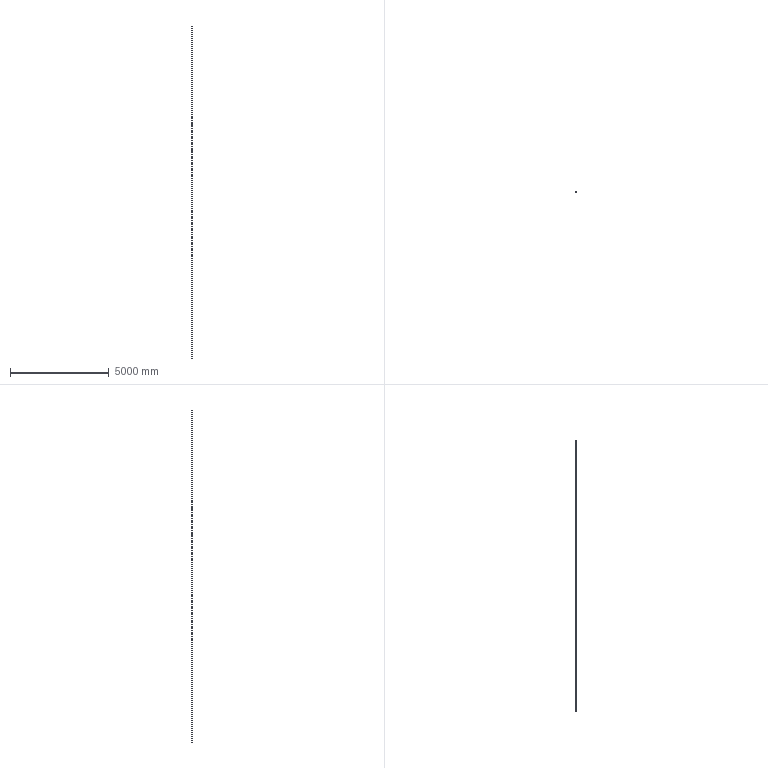Part | SolidWorks | features Extrusion 1 | 1 solid | 22 faces | box 32 x 30 x 16840 mm | volume 2880981 mm3 | plane 14 | cylinder 8 | commonest cylinder face diameters 8.4 x4 12 x4
STEP:
#1=CARTESIAN_POINT('',(-16.,-9.,0.));
#2=VERTEX_POINT('',#1);
#3=CARTESIAN_POINT('',(-10.,-15.,0.));
#4=VERTEX_POINT('',#3);
#5=CARTESIAN_POINT('',(-10.,-9.,0.));
#6=DIRECTION('',(0.,0.,1.));
#7=DIRECTION('',(1.,0.,0.));
#8=AXIS2_PLACEMENT_3D('',#5,#6,#7);
#9=CIRCLE('',#8,6.);
#10=EDGE_CURVE('',#2,#4,#9,.T.);
#11=ORIENTED_EDGE('',*,*,#10,.T.);
#12=CARTESIAN_POINT('',(-10.,-15.,16840.));
#13=VERTEX_POINT('',#12);
#14=CARTESIAN_POINT('',(-10.,-15.,16840.));
#15=DIRECTION('',(0.,0.,-1.));
#16=VECTOR('',#15,1000.);
#17=LINE('',#14,#16);
#18=EDGE_CURVE('',#13,#4,#17,.T.);
#19=ORIENTED_EDGE('',*,*,#18,.F.);
#20=CARTESIAN_POINT('',(-16.,-9.,16840.));
#21=VERTEX_POINT('',#20);
#22=CARTESIAN_POINT('',(-10.,-9.,16840.));
#23=DIRECTION('',(0.,0.,1.));
#24=DIRECTION('',(1.,0.,0.));
#25=AXIS2_PLACEMENT_3D('',#22,#23,#24);
#26=CIRCLE('',#25,6.);
#27=EDGE_CURVE('',#21,#13,#26,.T.);
#28=ORIENTED_EDGE('',*,*,#27,.F.);
#29=CARTESIAN_POINT('',(-16.,-9.,16840.));
#30=DIRECTION('',(0.,0.,-1.));
#31=VECTOR('',#30,1000.);
#32=LINE('',#29,#31);
#33=EDGE_CURVE('',#21,#2,#32,.T.);
#34=ORIENTED_EDGE('',*,*,#33,.T.);
#35=EDGE_LOOP('',(#11,#19,#28,#34));
#36=FACE_OUTER_BOUND('',#35,.T.);
#37=CARTESIAN_POINT('',(-10.,-9.,16840.));
#38=DIRECTION('',(0.,0.,-1.));
#39=DIRECTION('',(-1.,0.,0.));
#40=AXIS2_PLACEMENT_3D('',#37,#38,#39);
#41=CYLINDRICAL_SURFACE('',#40,6.);
#42=ADVANCED_FACE('',(#36),#41,.T.);
#43=CARTESIAN_POINT('',(-6.5,-15.,0.));
#44=VERTEX_POINT('',#43);
#45=CARTESIAN_POINT('',(-10.,-15.,0.));
#46=DIRECTION('',(1.,0.,0.));
#47=VECTOR('',#46,1000.);
#48=LINE('',#45,#47);
#49=EDGE_CURVE('',#4,#44,#48,.T.);
#50=ORIENTED_EDGE('',*,*,#49,.T.);
#51=CARTESIAN_POINT('',(-6.5,-15.,16840.));
#52=VERTEX_POINT('',#51);
#53=CARTESIAN_POINT('',(-6.5,-15.,16840.));
#54=DIRECTION('',(0.,0.,-1.));
#55=VECTOR('',#54,1000.);
#56=LINE('',#53,#55);
#57=EDGE_CURVE('',#52,#44,#56,.T.);
#58=ORIENTED_EDGE('',*,*,#57,.F.);
#59=CARTESIAN_POINT('',(-10.,-15.,16840.));
#60=DIRECTION('',(1.,0.,0.));
#61=VECTOR('',#60,1000.);
#62=LINE('',#59,#61);
#63=EDGE_CURVE('',#13,#52,#62,.T.);
#64=ORIENTED_EDGE('',*,*,#63,.F.);
#65=ORIENTED_EDGE('',*,*,#18,.T.);
#66=EDGE_LOOP('',(#50,#58,#64,#65));
#67=FACE_OUTER_BOUND('',#66,.T.);
#68=CARTESIAN_POINT('',(-10.,-15.,16840.));
#69=DIRECTION('',(0.,1.,0.));
#70=DIRECTION('',(-1.,0.,0.));
#71=AXIS2_PLACEMENT_3D('',#68,#69,#70);
#72=PLANE('',#71);
#73=ADVANCED_FACE('',(#67),#72,.F.);
#74=CARTESIAN_POINT('',(-6.5,-13.2,0.));
#75=VERTEX_POINT('',#74);
#76=CARTESIAN_POINT('',(-6.5,-15.,0.));
#77=DIRECTION('',(0.,1.,0.));
#78=VECTOR('',#77,1000.);
#79=LINE('',#76,#78);
#80=EDGE_CURVE('',#44,#75,#79,.T.);
#81=ORIENTED_EDGE('',*,*,#80,.T.);
#82=CARTESIAN_POINT('',(-6.5,-13.2,16840.));
#83=VERTEX_POINT('',#82);
#84=CARTESIAN_POINT('',(-6.5,-13.2,16840.));
#85=DIRECTION('',(0.,0.,-1.));
#86=VECTOR('',#85,1000.);
#87=LINE('',#84,#86);
#88=EDGE_CURVE('',#83,#75,#87,.T.);
#89=ORIENTED_EDGE('',*,*,#88,.F.);
#90=CARTESIAN_POINT('',(-6.5,-15.,16840.));
#91=DIRECTION('',(0.,1.,0.));
#92=VECTOR('',#91,1000.);
#93=LINE('',#90,#92);
#94=EDGE_CURVE('',#52,#83,#93,.T.);
#95=ORIENTED_EDGE('',*,*,#94,.F.);
#96=ORIENTED_EDGE('',*,*,#57,.T.);
#97=EDGE_LOOP('',(#81,#89,#95,#96));
#98=FACE_OUTER_BOUND('',#97,.T.);
#99=CARTESIAN_POINT('',(-6.5,-15.,16840.));
#100=DIRECTION('',(-1.,0.,0.));
#101=DIRECTION('',(0.,-1.,0.));
#102=AXIS2_PLACEMENT_3D('',#99,#100,#101);
#103=PLANE('',#102);
#104=ADVANCED_FACE('',(#98),#103,.F.);
#105=CARTESIAN_POINT('',(-10.,-13.2,0.));
#106=VERTEX_POINT('',#105);
#107=CARTESIAN_POINT('',(-10.,-13.2,0.));
#108=DIRECTION('',(-1.,0.,0.));
#109=VECTOR('',#108,1000.);
#110=LINE('',#107,#109);
#111=EDGE_CURVE('',#75,#106,#110,.T.);
#112=ORIENTED_EDGE('',*,*,#111,.T.);
#113=CARTESIAN_POINT('',(-10.,-13.2,16840.));
#114=VERTEX_POINT('',#113);
#115=CARTESIAN_POINT('',(-10.,-13.2,16840.));
#116=DIRECTION('',(0.,0.,-1.));
#117=VECTOR('',#116,1000.);
#118=LINE('',#115,#117);
#119=EDGE_CURVE('',#114,#106,#118,.T.);
#120=ORIENTED_EDGE('',*,*,#119,.F.);
#121=CARTESIAN_POINT('',(-10.,-13.2,16840.));
#122=DIRECTION('',(-1.,0.,0.));
#123=VECTOR('',#122,1000.);
#124=LINE('',#121,#123);
#125=EDGE_CURVE('',#83,#114,#124,.T.);
#126=ORIENTED_EDGE('',*,*,#125,.F.);
#127=ORIENTED_EDGE('',*,*,#88,.T.);
#128=EDGE_LOOP('',(#112,#120,#126,#127));
#129=FACE_OUTER_BOUND('',#128,.T.);
#130=CARTESIAN_POINT('',(-10.,-13.2,16840.));
#131=DIRECTION('',(0.,-1.,0.));
#132=DIRECTION('',(0.,0.,-1.));
#133=AXIS2_PLACEMENT_3D('',#130,#131,#132);
#134=PLANE('',#133);
#135=ADVANCED_FACE('',(#129),#134,.F.);
#136=CARTESIAN_POINT('',(-14.2,-9.,0.));
#137=VERTEX_POINT('',#136);
#138=CARTESIAN_POINT('',(-10.,-9.,0.));
#139=DIRECTION('',(0.,0.,-1.));
#140=DIRECTION('',(1.,0.,0.));
#141=AXIS2_PLACEMENT_3D('',#138,#139,#140);
#142=CIRCLE('',#141,4.2);
#143=EDGE_CURVE('',#106,#137,#142,.T.);
#144=ORIENTED_EDGE('',*,*,#143,.T.);
#145=CARTESIAN_POINT('',(-14.2,-9.,16840.));
#146=VERTEX_POINT('',#145);
#147=CARTESIAN_POINT('',(-14.2,-9.,16840.));
#148=DIRECTION('',(0.,0.,-1.));
#149=VECTOR('',#148,1000.);
#150=LINE('',#147,#149);
#151=EDGE_CURVE('',#146,#137,#150,.T.);
#152=ORIENTED_EDGE('',*,*,#151,.F.);
#153=CARTESIAN_POINT('',(-10.,-9.,16840.));
#154=DIRECTION('',(0.,0.,-1.));
#155=DIRECTION('',(1.,0.,0.));
#156=AXIS2_PLACEMENT_3D('',#153,#154,#155);
#157=CIRCLE('',#156,4.2);
#158=EDGE_CURVE('',#114,#146,#157,.T.);
#159=ORIENTED_EDGE('',*,*,#158,.F.);
#160=ORIENTED_EDGE('',*,*,#119,.T.);
#161=EDGE_LOOP('',(#144,#152,#159,#160));
#162=FACE_OUTER_BOUND('',#161,.T.);
#163=CARTESIAN_POINT('',(-10.,-9.,16840.));
#164=DIRECTION('',(0.,0.,-1.));
#165=DIRECTION('',(-1.,0.,0.));
#166=AXIS2_PLACEMENT_3D('',#163,#164,#165);
#167=CYLINDRICAL_SURFACE('',#166,4.2);
#168=ADVANCED_FACE('',(#162),#167,.F.);
#169=CARTESIAN_POINT('',(-14.2,9.,0.));
#170=VERTEX_POINT('',#169);
#171=CARTESIAN_POINT('',(-14.2,9.,0.));
#172=DIRECTION('',(0.,1.,0.));
#173=VECTOR('',#172,1000.);
#174=LINE('',#171,#173);
#175=EDGE_CURVE('',#137,#170,#174,.T.);
#176=ORIENTED_EDGE('',*,*,#175,.T.);
#177=CARTESIAN_POINT('',(-14.2,9.,16840.));
#178=VERTEX_POINT('',#177);
#179=CARTESIAN_POINT('',(-14.2,9.,16840.));
#180=DIRECTION('',(0.,0.,-1.));
#181=VECTOR('',#180,1000.);
#182=LINE('',#179,#181);
#183=EDGE_CURVE('',#178,#170,#182,.T.);
#184=ORIENTED_EDGE('',*,*,#183,.F.);
#185=CARTESIAN_POINT('',(-14.2,9.,16840.));
#186=DIRECTION('',(0.,1.,0.));
#187=VECTOR('',#186,1000.);
#188=LINE('',#185,#187);
#189=EDGE_CURVE('',#146,#178,#188,.T.);
#190=ORIENTED_EDGE('',*,*,#189,.F.);
#191=ORIENTED_EDGE('',*,*,#151,.T.);
#192=EDGE_LOOP('',(#176,#184,#190,#191));
#193=FACE_OUTER_BOUND('',#192,.T.);
#194=CARTESIAN_POINT('',(-14.2,9.,16840.));
#195=DIRECTION('',(-1.,0.,0.));
#196=DIRECTION('',(0.,0.,1.));
#197=AXIS2_PLACEMENT_3D('',#194,#195,#196);
#198=PLANE('',#197);
#199=ADVANCED_FACE('',(#193),#198,.F.);
#200=CARTESIAN_POINT('',(-10.,13.2,0.));
#201=VERTEX_POINT('',#200);
#202=CARTESIAN_POINT('',(-10.,9.,0.));
#203=DIRECTION('',(0.,0.,-1.));
#204=DIRECTION('',(1.,0.,0.));
#205=AXIS2_PLACEMENT_3D('',#202,#203,#204);
#206=CIRCLE('',#205,4.2);
#207=EDGE_CURVE('',#170,#201,#206,.T.);
#208=ORIENTED_EDGE('',*,*,#207,.T.);
#209=CARTESIAN_POINT('',(-10.,13.2,16840.));
#210=VERTEX_POINT('',#209);
#211=CARTESIAN_POINT('',(-10.,13.2,16840.));
#212=DIRECTION('',(0.,0.,-1.));
#213=VECTOR('',#212,1000.);
#214=LINE('',#211,#213);
#215=EDGE_CURVE('',#210,#201,#214,.T.);
#216=ORIENTED_EDGE('',*,*,#215,.F.);
#217=CARTESIAN_POINT('',(-10.,9.,16840.));
#218=DIRECTION('',(0.,0.,-1.));
#219=DIRECTION('',(1.,0.,0.));
#220=AXIS2_PLACEMENT_3D('',#217,#218,#219);
#221=CIRCLE('',#220,4.2);
#222=EDGE_CURVE('',#178,#210,#221,.T.);
#223=ORIENTED_EDGE('',*,*,#222,.F.);
#224=ORIENTED_EDGE('',*,*,#183,.T.);
#225=EDGE_LOOP('',(#208,#216,#223,#224));
#226=FACE_OUTER_BOUND('',#225,.T.);
#227=CARTESIAN_POINT('',(-10.,9.,16840.));
#228=DIRECTION('',(0.,0.,-1.));
#229=DIRECTION('',(-1.,0.,0.));
#230=AXIS2_PLACEMENT_3D('',#227,#228,#229);
#231=CYLINDRICAL_SURFACE('',#230,4.2);
#232=ADVANCED_FACE('',(#226),#231,.F.);
#233=CARTESIAN_POINT('',(10.,13.2,0.));
#234=VERTEX_POINT('',#233);
#235=CARTESIAN_POINT('',(-10.,13.2,0.));
#236=DIRECTION('',(1.,0.,0.));
#237=VECTOR('',#236,1000.);
#238=LINE('',#235,#237);
#239=EDGE_CURVE('',#201,#234,#238,.T.);
#240=ORIENTED_EDGE('',*,*,#239,.T.);
#241=CARTESIAN_POINT('',(10.,13.2,16840.));
#242=VERTEX_POINT('',#241);
#243=CARTESIAN_POINT('',(10.,13.2,16840.));
#244=DIRECTION('',(0.,0.,-1.));
#245=VECTOR('',#244,1000.);
#246=LINE('',#243,#245);
#247=EDGE_CURVE('',#242,#234,#246,.T.);
#248=ORIENTED_EDGE('',*,*,#247,.F.);
#249=CARTESIAN_POINT('',(-10.,13.2,16840.));
#250=DIRECTION('',(1.,0.,0.));
#251=VECTOR('',#250,1000.);
#252=LINE('',#249,#251);
#253=EDGE_CURVE('',#210,#242,#252,.T.);
#254=ORIENTED_EDGE('',*,*,#253,.F.);
#255=ORIENTED_EDGE('',*,*,#215,.T.);
#256=EDGE_LOOP('',(#240,#248,#254,#255));
#257=FACE_OUTER_BOUND('',#256,.T.);
#258=CARTESIAN_POINT('',(-10.,13.2,16840.));
#259=DIRECTION('',(0.,1.,0.));
#260=DIRECTION('',(-1.,0.,0.));
#261=AXIS2_PLACEMENT_3D('',#258,#259,#260);
#262=PLANE('',#261);
#263=ADVANCED_FACE('',(#257),#262,.F.);
#264=CARTESIAN_POINT('',(14.2,9.,0.));
#265=VERTEX_POINT('',#264);
#266=CARTESIAN_POINT('',(10.,9.,0.));
#267=DIRECTION('',(0.,0.,-1.));
#268=DIRECTION('',(-1.,0.,0.));
#269=AXIS2_PLACEMENT_3D('',#266,#267,#268);
#270=CIRCLE('',#269,4.2);
#271=EDGE_CURVE('',#234,#265,#270,.T.);
#272=ORIENTED_EDGE('',*,*,#271,.T.);
#273=CARTESIAN_POINT('',(14.2,9.,16840.));
#274=VERTEX_POINT('',#273);
#275=CARTESIAN_POINT('',(14.2,9.,16840.));
#276=DIRECTION('',(0.,0.,-1.));
#277=VECTOR('',#276,1000.);
#278=LINE('',#275,#277);
#279=EDGE_CURVE('',#274,#265,#278,.T.);
#280=ORIENTED_EDGE('',*,*,#279,.F.);
#281=CARTESIAN_POINT('',(10.,9.,16840.));
#282=DIRECTION('',(0.,0.,-1.));
#283=DIRECTION('',(-1.,0.,0.));
#284=AXIS2_PLACEMENT_3D('',#281,#282,#283);
#285=CIRCLE('',#284,4.2);
#286=EDGE_CURVE('',#242,#274,#285,.T.);
#287=ORIENTED_EDGE('',*,*,#286,.F.);
#288=ORIENTED_EDGE('',*,*,#247,.T.);
#289=EDGE_LOOP('',(#272,#280,#287,#288));
#290=FACE_OUTER_BOUND('',#289,.T.);
#291=CARTESIAN_POINT('',(10.,9.,16840.));
#292=DIRECTION('',(0.,0.,-1.));
#293=DIRECTION('',(-1.,0.,0.));
#294=AXIS2_PLACEMENT_3D('',#291,#292,#293);
#295=CYLINDRICAL_SURFACE('',#294,4.2);
#296=ADVANCED_FACE('',(#290),#295,.F.);
#297=CARTESIAN_POINT('',(14.2,-9.,0.));
#298=VERTEX_POINT('',#297);
#299=CARTESIAN_POINT('',(14.2,9.,0.));
#300=DIRECTION('',(0.,-1.,0.));
#301=VECTOR('',#300,1000.);
#302=LINE('',#299,#301);
#303=EDGE_CURVE('',#265,#298,#302,.T.);
#304=ORIENTED_EDGE('',*,*,#303,.T.);
#305=CARTESIAN_POINT('',(14.2,-9.,16840.));
#306=VERTEX_POINT('',#305);
#307=CARTESIAN_POINT('',(14.2,-9.,16840.));
#308=DIRECTION('',(0.,0.,-1.));
#309=VECTOR('',#308,1000.);
#310=LINE('',#307,#309);
#311=EDGE_CURVE('',#306,#298,#310,.T.);
#312=ORIENTED_EDGE('',*,*,#311,.F.);
#313=CARTESIAN_POINT('',(14.2,9.,16840.));
#314=DIRECTION('',(0.,-1.,0.));
#315=VECTOR('',#314,1000.);
#316=LINE('',#313,#315);
#317=EDGE_CURVE('',#274,#306,#316,.T.);
#318=ORIENTED_EDGE('',*,*,#317,.F.);
#319=ORIENTED_EDGE('',*,*,#279,.T.);
#320=EDGE_LOOP('',(#304,#312,#318,#319));
#321=FACE_OUTER_BOUND('',#320,.T.);
#322=CARTESIAN_POINT('',(14.2,9.,16840.));
#323=DIRECTION('',(1.,0.,0.));
#324=DIRECTION('',(0.,1.,0.));
#325=AXIS2_PLACEMENT_3D('',#322,#323,#324);
#326=PLANE('',#325);
#327=ADVANCED_FACE('',(#321),#326,.F.);
#328=CARTESIAN_POINT('',(10.,-13.2,0.));
#329=VERTEX_POINT('',#328);
#330=CARTESIAN_POINT('',(10.,-9.,0.));
#331=DIRECTION('',(0.,0.,-1.));
#332=DIRECTION('',(1.,0.,0.));
#333=AXIS2_PLACEMENT_3D('',#330,#331,#332);
#334=CIRCLE('',#333,4.2);
#335=EDGE_CURVE('',#298,#329,#334,.T.);
#336=ORIENTED_EDGE('',*,*,#335,.T.);
#337=CARTESIAN_POINT('',(10.,-13.2,16840.));
#338=VERTEX_POINT('',#337);
#339=CARTESIAN_POINT('',(10.,-13.2,16840.));
#340=DIRECTION('',(0.,0.,-1.));
#341=VECTOR('',#340,1000.);
#342=LINE('',#339,#341);
#343=EDGE_CURVE('',#338,#329,#342,.T.);
#344=ORIENTED_EDGE('',*,*,#343,.F.);
#345=CARTESIAN_POINT('',(10.,-9.,16840.));
#346=DIRECTION('',(0.,0.,-1.));
#347=DIRECTION('',(1.,0.,0.));
#348=AXIS2_PLACEMENT_3D('',#345,#346,#347);
#349=CIRCLE('',#348,4.2);
#350=EDGE_CURVE('',#306,#338,#349,.T.);
#351=ORIENTED_EDGE('',*,*,#350,.F.);
#352=ORIENTED_EDGE('',*,*,#311,.T.);
#353=EDGE_LOOP('',(#336,#344,#351,#352));
#354=FACE_OUTER_BOUND('',#353,.T.);
#355=CARTESIAN_POINT('',(10.,-9.,16840.));
#356=DIRECTION('',(0.,0.,-1.));
#357=DIRECTION('',(-1.,0.,0.));
#358=AXIS2_PLACEMENT_3D('',#355,#356,#357);
#359=CYLINDRICAL_SURFACE('',#358,4.2);
#360=ADVANCED_FACE('',(#354),#359,.F.);
#361=CARTESIAN_POINT('',(6.5,-13.2,0.));
#362=VERTEX_POINT('',#361);
#363=CARTESIAN_POINT('',(6.5,-13.2,0.));
#364=DIRECTION('',(-1.,0.,0.));
#365=VECTOR('',#364,1000.);
#366=LINE('',#363,#365);
#367=EDGE_CURVE('',#329,#362,#366,.T.);
#368=ORIENTED_EDGE('',*,*,#367,.T.);
#369=CARTESIAN_POINT('',(6.5,-13.2,16840.));
#370=VERTEX_POINT('',#369);
#371=CARTESIAN_POINT('',(6.5,-13.2,16840.));
#372=DIRECTION('',(0.,0.,-1.));
#373=VECTOR('',#372,1000.);
#374=LINE('',#371,#373);
#375=EDGE_CURVE('',#370,#362,#374,.T.);
#376=ORIENTED_EDGE('',*,*,#375,.F.);
#377=CARTESIAN_POINT('',(6.5,-13.2,16840.));
#378=DIRECTION('',(-1.,0.,0.));
#379=VECTOR('',#378,1000.);
#380=LINE('',#377,#379);
#381=EDGE_CURVE('',#338,#370,#380,.T.);
#382=ORIENTED_EDGE('',*,*,#381,.F.);
#383=ORIENTED_EDGE('',*,*,#343,.T.);
#384=EDGE_LOOP('',(#368,#376,#382,#383));
#385=FACE_OUTER_BOUND('',#384,.T.);
#386=CARTESIAN_POINT('',(6.5,-13.2,16840.));
#387=DIRECTION('',(0.,-1.,0.));
#388=DIRECTION('',(1.,0.,0.));
#389=AXIS2_PLACEMENT_3D('',#386,#387,#388);
#390=PLANE('',#389);
#391=ADVANCED_FACE('',(#385),#390,.F.);
#392=CARTESIAN_POINT('',(6.5,-15.,0.));
#393=VERTEX_POINT('',#392);
#394=CARTESIAN_POINT('',(6.5,-15.,0.));
#395=DIRECTION('',(0.,-1.,0.));
#396=VECTOR('',#395,1000.);
#397=LINE('',#394,#396);
#398=EDGE_CURVE('',#362,#393,#397,.T.);
#399=ORIENTED_EDGE('',*,*,#398,.T.);
#400=CARTESIAN_POINT('',(6.5,-15.,16840.));
#401=VERTEX_POINT('',#400);
#402=CARTESIAN_POINT('',(6.5,-15.,16840.));
#403=DIRECTION('',(0.,0.,-1.));
#404=VECTOR('',#403,1000.);
#405=LINE('',#402,#404);
#406=EDGE_CURVE('',#401,#393,#405,.T.);
#407=ORIENTED_EDGE('',*,*,#406,.F.);
#408=CARTESIAN_POINT('',(6.5,-15.,16840.));
#409=DIRECTION('',(0.,-1.,0.));
#410=VECTOR('',#409,1000.);
#411=LINE('',#408,#410);
#412=EDGE_CURVE('',#370,#401,#411,.T.);
#413=ORIENTED_EDGE('',*,*,#412,.F.);
#414=ORIENTED_EDGE('',*,*,#375,.T.);
#415=EDGE_LOOP('',(#399,#407,#413,#414));
#416=FACE_OUTER_BOUND('',#415,.T.);
#417=CARTESIAN_POINT('',(6.5,-15.,16840.));
#418=DIRECTION('',(1.,0.,0.));
#419=DIRECTION('',(0.,1.,0.));
#420=AXIS2_PLACEMENT_3D('',#417,#418,#419);
#421=PLANE('',#420);
#422=ADVANCED_FACE('',(#416),#421,.F.);
#423=CARTESIAN_POINT('',(10.,-15.,0.));
#424=VERTEX_POINT('',#423);
#425=CARTESIAN_POINT('',(6.5,-15.,0.));
#426=DIRECTION('',(1.,0.,0.));
#427=VECTOR('',#426,1000.);
#428=LINE('',#425,#427);
#429=EDGE_CURVE('',#393,#424,#428,.T.);
#430=ORIENTED_EDGE('',*,*,#429,.T.);
#431=CARTESIAN_POINT('',(10.,-15.,16840.));
#432=VERTEX_POINT('',#431);
#433=CARTESIAN_POINT('',(10.,-15.,16840.));
#434=DIRECTION('',(0.,0.,-1.));
#435=VECTOR('',#434,1000.);
#436=LINE('',#433,#435);
#437=EDGE_CURVE('',#432,#424,#436,.T.);
#438=ORIENTED_EDGE('',*,*,#437,.F.);
#439=CARTESIAN_POINT('',(6.5,-15.,16840.));
#440=DIRECTION('',(1.,0.,0.));
#441=VECTOR('',#440,1000.);
#442=LINE('',#439,#441);
#443=EDGE_CURVE('',#401,#432,#442,.T.);
#444=ORIENTED_EDGE('',*,*,#443,.F.);
#445=ORIENTED_EDGE('',*,*,#406,.T.);
#446=EDGE_LOOP('',(#430,#438,#444,#445));
#447=FACE_OUTER_BOUND('',#446,.T.);
#448=CARTESIAN_POINT('',(6.5,-15.,16840.));
#449=DIRECTION('',(0.,1.,0.));
#450=DIRECTION('',(0.,0.,1.));
#451=AXIS2_PLACEMENT_3D('',#448,#449,#450);
#452=PLANE('',#451);
#453=ADVANCED_FACE('',(#447),#452,.F.);
#454=CARTESIAN_POINT('',(16.,-9.,0.));
#455=VERTEX_POINT('',#454);
#456=CARTESIAN_POINT('',(10.,-9.,0.));
#457=DIRECTION('',(0.,0.,1.));
#458=DIRECTION('',(1.,0.,0.));
#459=AXIS2_PLACEMENT_3D('',#456,#457,#458);
#460=CIRCLE('',#459,6.);
#461=EDGE_CURVE('',#424,#455,#460,.T.);
#462=ORIENTED_EDGE('',*,*,#461,.T.);
#463=CARTESIAN_POINT('',(16.,-9.,16840.));
#464=VERTEX_POINT('',#463);
#465=CARTESIAN_POINT('',(16.,-9.,16840.));
#466=DIRECTION('',(0.,0.,-1.));
#467=VECTOR('',#466,1000.);
#468=LINE('',#465,#467);
#469=EDGE_CURVE('',#464,#455,#468,.T.);
#470=ORIENTED_EDGE('',*,*,#469,.F.);
#471=CARTESIAN_POINT('',(10.,-9.,16840.));
#472=DIRECTION('',(0.,0.,1.));
#473=DIRECTION('',(1.,0.,0.));
#474=AXIS2_PLACEMENT_3D('',#471,#472,#473);
#475=CIRCLE('',#474,6.);
#476=EDGE_CURVE('',#432,#464,#475,.T.);
#477=ORIENTED_EDGE('',*,*,#476,.F.);
#478=ORIENTED_EDGE('',*,*,#437,.T.);
#479=EDGE_LOOP('',(#462,#470,#477,#478));
#480=FACE_OUTER_BOUND('',#479,.T.);
#481=CARTESIAN_POINT('',(10.,-9.,16840.));
#482=DIRECTION('',(0.,0.,-1.));
#483=DIRECTION('',(-1.,0.,0.));
#484=AXIS2_PLACEMENT_3D('',#481,#482,#483);
#485=CYLINDRICAL_SURFACE('',#484,6.);
#486=ADVANCED_FACE('',(#480),#485,.T.);
#487=CARTESIAN_POINT('',(16.,9.,0.));
#488=VERTEX_POINT('',#487);
#489=CARTESIAN_POINT('',(16.,9.,0.));
#490=DIRECTION('',(0.,1.,0.));
#491=VECTOR('',#490,1000.);
#492=LINE('',#489,#491);
#493=EDGE_CURVE('',#455,#488,#492,.T.);
#494=ORIENTED_EDGE('',*,*,#493,.T.);
#495=CARTESIAN_POINT('',(16.,9.,16840.));
#496=VERTEX_POINT('',#495);
#497=CARTESIAN_POINT('',(16.,9.,16840.));
#498=DIRECTION('',(0.,0.,-1.));
#499=VECTOR('',#498,1000.);
#500=LINE('',#497,#499);
#501=EDGE_CURVE('',#496,#488,#500,.T.);
#502=ORIENTED_EDGE('',*,*,#501,.F.);
#503=CARTESIAN_POINT('',(16.,9.,16840.));
#504=DIRECTION('',(0.,1.,0.));
#505=VECTOR('',#504,1000.);
#506=LINE('',#503,#505);
#507=EDGE_CURVE('',#464,#496,#506,.T.);
#508=ORIENTED_EDGE('',*,*,#507,.F.);
#509=ORIENTED_EDGE('',*,*,#469,.T.);
#510=EDGE_LOOP('',(#494,#502,#508,#509));
#511=FACE_OUTER_BOUND('',#510,.T.);
#512=CARTESIAN_POINT('',(16.,9.,16840.));
#513=DIRECTION('',(-1.,0.,0.));
#514=DIRECTION('',(0.,-1.,0.));
#515=AXIS2_PLACEMENT_3D('',#512,#513,#514);
#516=PLANE('',#515);
#517=ADVANCED_FACE('',(#511),#516,.F.);
#518=CARTESIAN_POINT('',(10.,15.,0.));
#519=VERTEX_POINT('',#518);
#520=CARTESIAN_POINT('',(10.,9.,0.));
#521=DIRECTION('',(0.,0.,1.));
#522=DIRECTION('',(-1.,0.,0.));
#523=AXIS2_PLACEMENT_3D('',#520,#521,#522);
#524=CIRCLE('',#523,6.);
#525=EDGE_CURVE('',#488,#519,#524,.T.);
#526=ORIENTED_EDGE('',*,*,#525,.T.);
#527=CARTESIAN_POINT('',(10.,15.,16840.));
#528=VERTEX_POINT('',#527);
#529=CARTESIAN_POINT('',(10.,15.,16840.));
#530=DIRECTION('',(0.,0.,-1.));
#531=VECTOR('',#530,1000.);
#532=LINE('',#529,#531);
#533=EDGE_CURVE('',#528,#519,#532,.T.);
#534=ORIENTED_EDGE('',*,*,#533,.F.);
#535=CARTESIAN_POINT('',(10.,9.,16840.));
#536=DIRECTION('',(0.,0.,1.));
#537=DIRECTION('',(-1.,0.,0.));
#538=AXIS2_PLACEMENT_3D('',#535,#536,#537);
#539=CIRCLE('',#538,6.);
#540=EDGE_CURVE('',#496,#528,#539,.T.);
#541=ORIENTED_EDGE('',*,*,#540,.F.);
#542=ORIENTED_EDGE('',*,*,#501,.T.);
#543=EDGE_LOOP('',(#526,#534,#541,#542));
#544=FACE_OUTER_BOUND('',#543,.T.);
#545=CARTESIAN_POINT('',(10.,9.,16840.));
#546=DIRECTION('',(0.,0.,-1.));
#547=DIRECTION('',(-1.,0.,0.));
#548=AXIS2_PLACEMENT_3D('',#545,#546,#547);
#549=CYLINDRICAL_SURFACE('',#548,6.);
#550=ADVANCED_FACE('',(#544),#549,.T.);
#551=CARTESIAN_POINT('',(-10.,15.,0.));
#552=VERTEX_POINT('',#551);
#553=CARTESIAN_POINT('',(-10.,15.,0.));
#554=DIRECTION('',(-1.,0.,0.));
#555=VECTOR('',#554,1000.);
#556=LINE('',#553,#555);
#557=EDGE_CURVE('',#519,#552,#556,.T.);
#558=ORIENTED_EDGE('',*,*,#557,.T.);
#559=CARTESIAN_POINT('',(-10.,15.,16840.));
#560=VERTEX_POINT('',#559);
#561=CARTESIAN_POINT('',(-10.,15.,16840.));
#562=DIRECTION('',(0.,0.,-1.));
#563=VECTOR('',#562,1000.);
#564=LINE('',#561,#563);
#565=EDGE_CURVE('',#560,#552,#564,.T.);
#566=ORIENTED_EDGE('',*,*,#565,.F.);
#567=CARTESIAN_POINT('',(-10.,15.,16840.));
#568=DIRECTION('',(-1.,0.,0.));
#569=VECTOR('',#568,1000.);
#570=LINE('',#567,#569);
#571=EDGE_CURVE('',#528,#560,#570,.T.);
#572=ORIENTED_EDGE('',*,*,#571,.F.);
#573=ORIENTED_EDGE('',*,*,#533,.T.);
#574=EDGE_LOOP('',(#558,#566,#572,#573));
#575=FACE_OUTER_BOUND('',#574,.T.);
#576=CARTESIAN_POINT('',(-10.,15.,16840.));
#577=DIRECTION('',(0.,-1.,0.));
#578=DIRECTION('',(0.,0.,-1.));
#579=AXIS2_PLACEMENT_3D('',#576,#577,#578);
#580=PLANE('',#579);
#581=ADVANCED_FACE('',(#575),#580,.F.);
#582=CARTESIAN_POINT('',(-16.,9.,0.));
#583=VERTEX_POINT('',#582);
#584=CARTESIAN_POINT('',(-10.,9.,0.));
#585=DIRECTION('',(0.,0.,1.));
#586=DIRECTION('',(1.,0.,0.));
#587=AXIS2_PLACEMENT_3D('',#584,#585,#586);
#588=CIRCLE('',#587,6.);
#589=EDGE_CURVE('',#552,#583,#588,.T.);
#590=ORIENTED_EDGE('',*,*,#589,.T.);
#591=CARTESIAN_POINT('',(-16.,9.,16840.));
#592=VERTEX_POINT('',#591);
#593=CARTESIAN_POINT('',(-16.,9.,16840.));
#594=DIRECTION('',(0.,0.,-1.));
#595=VECTOR('',#594,1000.);
#596=LINE('',#593,#595);
#597=EDGE_CURVE('',#592,#583,#596,.T.);
#598=ORIENTED_EDGE('',*,*,#597,.F.);
#599=CARTESIAN_POINT('',(-10.,9.,16840.));
#600=DIRECTION('',(0.,0.,1.));
#601=DIRECTION('',(1.,0.,0.));
#602=AXIS2_PLACEMENT_3D('',#599,#600,#601);
#603=CIRCLE('',#602,6.);
#604=EDGE_CURVE('',#560,#592,#603,.T.);
#605=ORIENTED_EDGE('',*,*,#604,.F.);
#606=ORIENTED_EDGE('',*,*,#565,.T.);
#607=EDGE_LOOP('',(#590,#598,#605,#606));
#608=FACE_OUTER_BOUND('',#607,.T.);
#609=CARTESIAN_POINT('',(-10.,9.,16840.));
#610=DIRECTION('',(0.,0.,-1.));
#611=DIRECTION('',(-1.,0.,0.));
#612=AXIS2_PLACEMENT_3D('',#609,#610,#611);
#613=CYLINDRICAL_SURFACE('',#612,6.);
#614=ADVANCED_FACE('',(#608),#613,.T.);
#615=CARTESIAN_POINT('',(-16.,9.,0.));
#616=DIRECTION('',(0.,-1.,0.));
#617=VECTOR('',#616,1000.);
#618=LINE('',#615,#617);
#619=EDGE_CURVE('',#583,#2,#618,.T.);
#620=ORIENTED_EDGE('',*,*,#619,.T.);
#621=ORIENTED_EDGE('',*,*,#33,.F.);
#622=CARTESIAN_POINT('',(-16.,9.,16840.));
#623=DIRECTION('',(0.,-1.,0.));
#624=VECTOR('',#623,1000.);
#625=LINE('',#622,#624);
#626=EDGE_CURVE('',#592,#21,#625,.T.);
#627=ORIENTED_EDGE('',*,*,#626,.F.);
#628=ORIENTED_EDGE('',*,*,#597,.T.);
#629=EDGE_LOOP('',(#620,#621,#627,#628));
#630=FACE_OUTER_BOUND('',#629,.T.);
#631=CARTESIAN_POINT('',(-16.,9.,16840.));
#632=DIRECTION('',(1.,0.,0.));
#633=DIRECTION('',(0.,0.,-1.));
#634=AXIS2_PLACEMENT_3D('',#631,#632,#633);
#635=PLANE('',#634);
#636=ADVANCED_FACE('',(#630),#635,.F.);
#637=ORIENTED_EDGE('',*,*,#27,.T.);
#638=ORIENTED_EDGE('',*,*,#63,.T.);
#639=ORIENTED_EDGE('',*,*,#94,.T.);
#640=ORIENTED_EDGE('',*,*,#125,.T.);
#641=ORIENTED_EDGE('',*,*,#158,.T.);
#642=ORIENTED_EDGE('',*,*,#189,.T.);
#643=ORIENTED_EDGE('',*,*,#222,.T.);
#644=ORIENTED_EDGE('',*,*,#253,.T.);
#645=ORIENTED_EDGE('',*,*,#286,.T.);
#646=ORIENTED_EDGE('',*,*,#317,.T.);
#647=ORIENTED_EDGE('',*,*,#350,.T.);
#648=ORIENTED_EDGE('',*,*,#381,.T.);
#649=ORIENTED_EDGE('',*,*,#412,.T.);
#650=ORIENTED_EDGE('',*,*,#443,.T.);
#651=ORIENTED_EDGE('',*,*,#476,.T.);
#652=ORIENTED_EDGE('',*,*,#507,.T.);
#653=ORIENTED_EDGE('',*,*,#540,.T.);
#654=ORIENTED_EDGE('',*,*,#571,.T.);
#655=ORIENTED_EDGE('',*,*,#604,.T.);
#656=ORIENTED_EDGE('',*,*,#626,.T.);
#657=EDGE_LOOP('',(#637,#638,#639,#640,#641,#642,#643,#644,#645,#646,#647,#648,#649,#650,#651,#652,#653,#654,#655,#656));
#658=FACE_OUTER_BOUND('',#657,.T.);
#659=CARTESIAN_POINT('',(-10.,-9.,16840.));
#660=DIRECTION('',(0.,0.,1.));
#661=DIRECTION('',(1.,0.,0.));
#662=AXIS2_PLACEMENT_3D('',#659,#660,#661);
#663=PLANE('',#662);
#664=ADVANCED_FACE('',(#658),#663,.T.);
#665=ORIENTED_EDGE('',*,*,#10,.F.);
#666=ORIENTED_EDGE('',*,*,#619,.F.);
#667=ORIENTED_EDGE('',*,*,#589,.F.);
#668=ORIENTED_EDGE('',*,*,#557,.F.);
#669=ORIENTED_EDGE('',*,*,#525,.F.);
#670=ORIENTED_EDGE('',*,*,#493,.F.);
#671=ORIENTED_EDGE('',*,*,#461,.F.);
#672=ORIENTED_EDGE('',*,*,#429,.F.);
#673=ORIENTED_EDGE('',*,*,#398,.F.);
#674=ORIENTED_EDGE('',*,*,#367,.F.);
#675=ORIENTED_EDGE('',*,*,#335,.F.);
#676=ORIENTED_EDGE('',*,*,#303,.F.);
#677=ORIENTED_EDGE('',*,*,#271,.F.);
#678=ORIENTED_EDGE('',*,*,#239,.F.);
#679=ORIENTED_EDGE('',*,*,#207,.F.);
#680=ORIENTED_EDGE('',*,*,#175,.F.);
#681=ORIENTED_EDGE('',*,*,#143,.F.);
#682=ORIENTED_EDGE('',*,*,#111,.F.);
#683=ORIENTED_EDGE('',*,*,#80,.F.);
#684=ORIENTED_EDGE('',*,*,#49,.F.);
#685=EDGE_LOOP('',(#665,#666,#667,#668,#669,#670,#671,#672,#673,#674,#675,#676,#677,#678,#679,#680,#681,#682,#683,#684));
#686=FACE_OUTER_BOUND('',#685,.T.);
#687=CARTESIAN_POINT('',(-10.,-9.,0.));
#688=DIRECTION('',(0.,0.,1.));
#689=DIRECTION('',(1.,0.,0.));
#690=AXIS2_PLACEMENT_3D('',#687,#688,#689);
#691=PLANE('',#690);
#692=ADVANCED_FACE('',(#686),#691,.F.);
#693=CLOSED_SHELL('',(#42,#73,#104,#135,#168,#199,#232,#263,#296,#327,#360,#391,#422,#453,#486,#517,#550,#581,#614,#636,#664,#692));
#694=MANIFOLD_SOLID_BREP('',#693);
#695=CARTESIAN_POINT('',(0.,0.,0.));
#696=DIRECTION('',(0.,0.,1.));
#697=DIRECTION('',(1.,0.,0.));
#698=AXIS2_PLACEMENT_3D('',#695,#696,#697);
#699=(LENGTH_UNIT()NAMED_UNIT(*)SI_UNIT(.MILLI.,.METRE.));
#700=UNCERTAINTY_MEASURE_WITH_UNIT(LENGTH_MEASURE(0.00001),#699,'','');
#701=(NAMED_UNIT(*)PLANE_ANGLE_UNIT()SI_UNIT($,.RADIAN.));
#702=(NAMED_UNIT(*)SI_UNIT($,.STERADIAN.)SOLID_ANGLE_UNIT());
#703=(GEOMETRIC_REPRESENTATION_CONTEXT(3)GLOBAL_UNCERTAINTY_ASSIGNED_CONTEXT((#700))GLOBAL_UNIT_ASSIGNED_CONTEXT((#699,#701,#702))REPRESENTATION_CONTEXT('',''));
#704=ADVANCED_BREP_SHAPE_REPRESENTATION('',(#694,#698),#703);